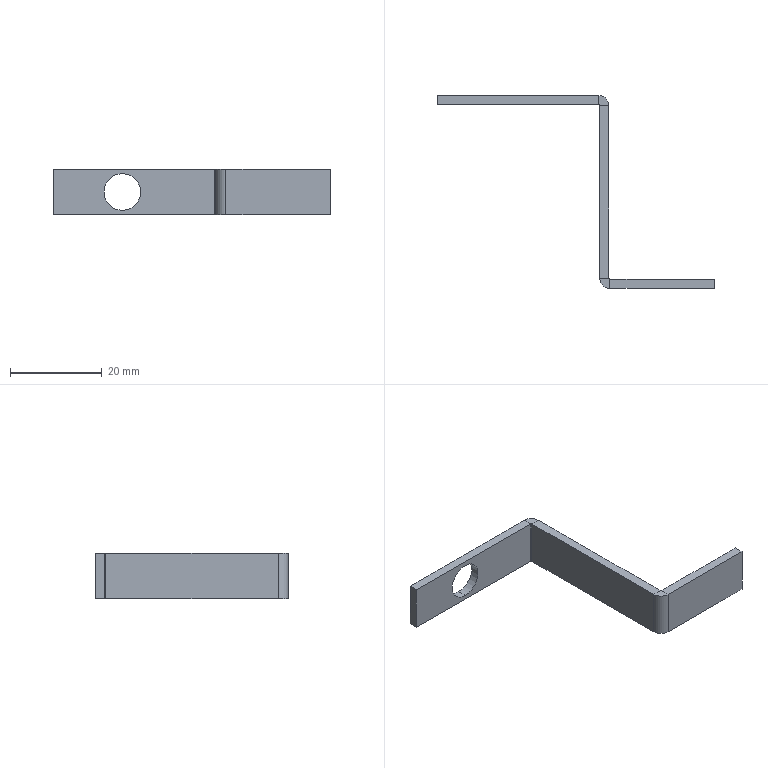Part | STEP file | Sensor support | 1 solid | 24 faces | box 60.39 x 42 x 10 mm | volume 1887 mm3 | plane 18 | cylinder 6 | commonest cylinder face diameters 0.4 x2 4.4 x2 8 x2
STEP:
#1=CARTESIAN_POINT('',(-45.39,40.,-4.));
#2=VERTEX_POINT('',#1);
#3=CARTESIAN_POINT('',(-45.39,40.,4.));
#4=VERTEX_POINT('',#3);
#5=CARTESIAN_POINT('',(-45.39,40.,0.));
#6=DIRECTION('',(0.,1.,0.));
#7=DIRECTION('',(1.,0.,0.));
#8=AXIS2_PLACEMENT_3D('',#5,#6,#7);
#9=CIRCLE('',#8,4.);
#10=EDGE_CURVE('',#2,#4,#9,.T.);
#11=ORIENTED_EDGE('',*,*,#10,.F.);
#12=CARTESIAN_POINT('',(-45.39,42.,-4.));
#13=VERTEX_POINT('',#12);
#14=CARTESIAN_POINT('',(-45.39,-0.001,-4.));
#15=DIRECTION('',(0.,1.,0.));
#16=VECTOR('',#15,1000.);
#17=LINE('',#14,#16);
#18=EDGE_CURVE('',#2,#13,#17,.T.);
#19=ORIENTED_EDGE('',*,*,#18,.T.);
#20=CARTESIAN_POINT('',(-45.39,42.,4.));
#21=VERTEX_POINT('',#20);
#22=CARTESIAN_POINT('',(-45.39,42.,0.));
#23=DIRECTION('',(0.,1.,0.));
#24=DIRECTION('',(0.,0.,1.));
#25=AXIS2_PLACEMENT_3D('',#22,#23,#24);
#26=CIRCLE('',#25,4.);
#27=EDGE_CURVE('',#13,#21,#26,.T.);
#28=ORIENTED_EDGE('',*,*,#27,.T.);
#29=CARTESIAN_POINT('',(-45.39,-0.001,4.));
#30=DIRECTION('',(0.,1.,0.));
#31=VECTOR('',#30,1000.);
#32=LINE('',#29,#31);
#33=EDGE_CURVE('',#4,#21,#32,.T.);
#34=ORIENTED_EDGE('',*,*,#33,.F.);
#35=EDGE_LOOP('',(#11,#19,#28,#34));
#36=FACE_OUTER_BOUND('',#35,.T.);
#37=CARTESIAN_POINT('',(-45.39,-0.001,0.));
#38=DIRECTION('',(0.,1.,0.));
#39=DIRECTION('',(0.,0.,1.));
#40=AXIS2_PLACEMENT_3D('',#37,#38,#39);
#41=CYLINDRICAL_SURFACE('',#40,4.);
#42=ADVANCED_FACE('',(#36),#41,.F.);
#43=CARTESIAN_POINT('',(-25.,2.2,5.));
#44=VERTEX_POINT('',#43);
#45=CARTESIAN_POINT('',(-23.,2.2,5.));
#46=VERTEX_POINT('',#45);
#47=CARTESIAN_POINT('',(-25.,2.2,5.));
#48=DIRECTION('',(1.,0.,0.));
#49=VECTOR('',#48,1000.);
#50=LINE('',#47,#49);
#51=EDGE_CURVE('',#44,#46,#50,.T.);
#52=ORIENTED_EDGE('',*,*,#51,.F.);
#53=CARTESIAN_POINT('',(-22.8,0.,5.));
#54=VERTEX_POINT('',#53);
#55=CARTESIAN_POINT('',(-22.8,2.2,5.));
#56=DIRECTION('',(0.,0.,-1.));
#57=DIRECTION('',(1.,0.,0.));
#58=AXIS2_PLACEMENT_3D('',#55,#56,#57);
#59=CIRCLE('',#58,2.2);
#60=EDGE_CURVE('',#54,#44,#59,.T.);
#61=ORIENTED_EDGE('',*,*,#60,.F.);
#62=CARTESIAN_POINT('',(-22.8,2.,5.));
#63=VERTEX_POINT('',#62);
#64=CARTESIAN_POINT('',(-22.8,2.,5.));
#65=DIRECTION('',(0.,-1.,0.));
#66=VECTOR('',#65,1000.);
#67=LINE('',#64,#66);
#68=EDGE_CURVE('',#63,#54,#67,.T.);
#69=ORIENTED_EDGE('',*,*,#68,.F.);
#70=CARTESIAN_POINT('',(-22.8,2.2,5.));
#71=DIRECTION('',(0.,0.,-1.));
#72=DIRECTION('',(1.,0.,0.));
#73=AXIS2_PLACEMENT_3D('',#70,#71,#72);
#74=CIRCLE('',#73,0.2);
#75=EDGE_CURVE('',#63,#46,#74,.T.);
#76=ORIENTED_EDGE('',*,*,#75,.T.);
#77=EDGE_LOOP('',(#52,#61,#69,#76));
#78=FACE_OUTER_BOUND('',#77,.T.);
#79=CARTESIAN_POINT('',(-25.,2.2,5.));
#80=DIRECTION('',(0.,0.,1.));
#81=DIRECTION('',(1.,0.,0.));
#82=AXIS2_PLACEMENT_3D('',#79,#80,#81);
#83=PLANE('',#82);
#84=ADVANCED_FACE('',(#78),#83,.T.);
#85=CARTESIAN_POINT('',(-25.,39.8,5.));
#86=VERTEX_POINT('',#85);
#87=CARTESIAN_POINT('',(-25.,0.,5.));
#88=DIRECTION('',(0.,1.,0.));
#89=VECTOR('',#88,1000.);
#90=LINE('',#87,#89);
#91=EDGE_CURVE('',#44,#86,#90,.T.);
#92=ORIENTED_EDGE('',*,*,#91,.F.);
#93=ORIENTED_EDGE('',*,*,#51,.T.);
#94=CARTESIAN_POINT('',(-23.,39.8,5.));
#95=VERTEX_POINT('',#94);
#96=CARTESIAN_POINT('',(-23.,0.,5.));
#97=DIRECTION('',(0.,1.,0.));
#98=VECTOR('',#97,1000.);
#99=LINE('',#96,#98);
#100=EDGE_CURVE('',#46,#95,#99,.T.);
#101=ORIENTED_EDGE('',*,*,#100,.T.);
#102=CARTESIAN_POINT('',(-23.,39.8,5.));
#103=DIRECTION('',(-1.,0.,0.));
#104=VECTOR('',#103,1000.);
#105=LINE('',#102,#104);
#106=EDGE_CURVE('',#95,#86,#105,.T.);
#107=ORIENTED_EDGE('',*,*,#106,.T.);
#108=EDGE_LOOP('',(#92,#93,#101,#107));
#109=FACE_OUTER_BOUND('',#108,.T.);
#110=CARTESIAN_POINT('',(-22.8,2.,5.));
#111=DIRECTION('',(0.,0.,1.));
#112=DIRECTION('',(1.,0.,0.));
#113=AXIS2_PLACEMENT_3D('',#110,#111,#112);
#114=PLANE('',#113);
#115=ADVANCED_FACE('',(#109),#114,.T.);
#116=CARTESIAN_POINT('',(-22.8,0.,-5.));
#117=VERTEX_POINT('',#116);
#118=CARTESIAN_POINT('',(-22.8,2.,-5.));
#119=VERTEX_POINT('',#118);
#120=CARTESIAN_POINT('',(-22.8,0.,-5.));
#121=DIRECTION('',(0.,1.,0.));
#122=VECTOR('',#121,1000.);
#123=LINE('',#120,#122);
#124=EDGE_CURVE('',#117,#119,#123,.T.);
#125=ORIENTED_EDGE('',*,*,#124,.F.);
#126=CARTESIAN_POINT('',(-25.,2.2,-5.));
#127=VERTEX_POINT('',#126);
#128=CARTESIAN_POINT('',(-22.8,2.2,-5.));
#129=DIRECTION('',(0.,0.,-1.));
#130=DIRECTION('',(1.,0.,0.));
#131=AXIS2_PLACEMENT_3D('',#128,#129,#130);
#132=CIRCLE('',#131,2.2);
#133=EDGE_CURVE('',#117,#127,#132,.T.);
#134=ORIENTED_EDGE('',*,*,#133,.T.);
#135=CARTESIAN_POINT('',(-23.,2.2,-5.));
#136=VERTEX_POINT('',#135);
#137=CARTESIAN_POINT('',(-23.,2.2,-5.));
#138=DIRECTION('',(-1.,0.,0.));
#139=VECTOR('',#138,1000.);
#140=LINE('',#137,#139);
#141=EDGE_CURVE('',#136,#127,#140,.T.);
#142=ORIENTED_EDGE('',*,*,#141,.F.);
#143=CARTESIAN_POINT('',(-22.8,2.2,-5.));
#144=DIRECTION('',(0.,0.,-1.));
#145=DIRECTION('',(1.,0.,0.));
#146=AXIS2_PLACEMENT_3D('',#143,#144,#145);
#147=CIRCLE('',#146,0.2);
#148=EDGE_CURVE('',#119,#136,#147,.T.);
#149=ORIENTED_EDGE('',*,*,#148,.F.);
#150=EDGE_LOOP('',(#125,#134,#142,#149));
#151=FACE_OUTER_BOUND('',#150,.T.);
#152=CARTESIAN_POINT('',(-22.8,0.,-5.));
#153=DIRECTION('',(0.,0.,-1.));
#154=DIRECTION('',(-1.,0.,0.));
#155=AXIS2_PLACEMENT_3D('',#152,#153,#154);
#156=PLANE('',#155);
#157=ADVANCED_FACE('',(#151),#156,.T.);
#158=CARTESIAN_POINT('',(0.,0.,-5.));
#159=VERTEX_POINT('',#158);
#160=CARTESIAN_POINT('',(0.,0.,-5.));
#161=DIRECTION('',(-1.,0.,0.));
#162=VECTOR('',#161,1000.);
#163=LINE('',#160,#162);
#164=EDGE_CURVE('',#159,#117,#163,.T.);
#165=ORIENTED_EDGE('',*,*,#164,.T.);
#166=ORIENTED_EDGE('',*,*,#124,.T.);
#167=CARTESIAN_POINT('',(0.,2.,-5.));
#168=VERTEX_POINT('',#167);
#169=CARTESIAN_POINT('',(0.,2.,-5.));
#170=DIRECTION('',(-1.,0.,0.));
#171=VECTOR('',#170,1000.);
#172=LINE('',#169,#171);
#173=EDGE_CURVE('',#168,#119,#172,.T.);
#174=ORIENTED_EDGE('',*,*,#173,.F.);
#175=CARTESIAN_POINT('',(0.,2.,-5.));
#176=DIRECTION('',(0.,-1.,0.));
#177=VECTOR('',#176,1000.);
#178=LINE('',#175,#177);
#179=EDGE_CURVE('',#168,#159,#178,.T.);
#180=ORIENTED_EDGE('',*,*,#179,.T.);
#181=EDGE_LOOP('',(#165,#166,#174,#180));
#182=FACE_OUTER_BOUND('',#181,.T.);
#183=CARTESIAN_POINT('',(-23.,2.2,-5.));
#184=DIRECTION('',(0.,0.,-1.));
#185=DIRECTION('',(-1.,0.,0.));
#186=AXIS2_PLACEMENT_3D('',#183,#184,#185);
#187=PLANE('',#186);
#188=ADVANCED_FACE('',(#182),#187,.T.);
#189=CARTESIAN_POINT('',(-25.2,40.,5.));
#190=VERTEX_POINT('',#189);
#191=CARTESIAN_POINT('',(-25.2,42.,5.));
#192=VERTEX_POINT('',#191);
#193=CARTESIAN_POINT('',(-25.2,40.,5.));
#194=DIRECTION('',(0.,1.,0.));
#195=VECTOR('',#194,1000.);
#196=LINE('',#193,#195);
#197=EDGE_CURVE('',#190,#192,#196,.T.);
#198=ORIENTED_EDGE('',*,*,#197,.F.);
#199=CARTESIAN_POINT('',(-25.2,39.8,5.));
#200=DIRECTION('',(0.,0.,1.));
#201=DIRECTION('',(-1.,0.,0.));
#202=AXIS2_PLACEMENT_3D('',#199,#200,#201);
#203=CIRCLE('',#202,0.2);
#204=EDGE_CURVE('',#86,#190,#203,.T.);
#205=ORIENTED_EDGE('',*,*,#204,.F.);
#206=ORIENTED_EDGE('',*,*,#106,.F.);
#207=CARTESIAN_POINT('',(-25.2,39.8,5.));
#208=DIRECTION('',(0.,0.,1.));
#209=DIRECTION('',(1.,0.,0.));
#210=AXIS2_PLACEMENT_3D('',#207,#208,#209);
#211=CIRCLE('',#210,2.2);
#212=EDGE_CURVE('',#95,#192,#211,.T.);
#213=ORIENTED_EDGE('',*,*,#212,.T.);
#214=EDGE_LOOP('',(#198,#205,#206,#213));
#215=FACE_OUTER_BOUND('',#214,.T.);
#216=CARTESIAN_POINT('',(-25.2,40.,5.));
#217=DIRECTION('',(0.,0.,1.));
#218=DIRECTION('',(1.,0.,0.));
#219=AXIS2_PLACEMENT_3D('',#216,#217,#218);
#220=PLANE('',#219);
#221=ADVANCED_FACE('',(#215),#220,.T.);
#222=CARTESIAN_POINT('',(-60.39,40.,5.));
#223=VERTEX_POINT('',#222);
#224=CARTESIAN_POINT('',(-25.,40.,5.));
#225=DIRECTION('',(-1.,0.,0.));
#226=VECTOR('',#225,1000.);
#227=LINE('',#224,#226);
#228=EDGE_CURVE('',#190,#223,#227,.T.);
#229=ORIENTED_EDGE('',*,*,#228,.F.);
#230=ORIENTED_EDGE('',*,*,#197,.T.);
#231=CARTESIAN_POINT('',(-60.39,42.,5.));
#232=VERTEX_POINT('',#231);
#233=CARTESIAN_POINT('',(-25.,42.,5.));
#234=DIRECTION('',(-1.,0.,0.));
#235=VECTOR('',#234,1000.);
#236=LINE('',#233,#235);
#237=EDGE_CURVE('',#192,#232,#236,.T.);
#238=ORIENTED_EDGE('',*,*,#237,.T.);
#239=CARTESIAN_POINT('',(-60.39,40.,5.));
#240=DIRECTION('',(0.,1.,0.));
#241=VECTOR('',#240,1000.);
#242=LINE('',#239,#241);
#243=EDGE_CURVE('',#223,#232,#242,.T.);
#244=ORIENTED_EDGE('',*,*,#243,.F.);
#245=EDGE_LOOP('',(#229,#230,#238,#244));
#246=FACE_OUTER_BOUND('',#245,.T.);
#247=CARTESIAN_POINT('',(-23.,39.8,5.));
#248=DIRECTION('',(0.,0.,1.));
#249=DIRECTION('',(1.,0.,0.));
#250=AXIS2_PLACEMENT_3D('',#247,#248,#249);
#251=PLANE('',#250);
#252=ADVANCED_FACE('',(#246),#251,.T.);
#253=CARTESIAN_POINT('',(-25.,39.8,-5.));
#254=VERTEX_POINT('',#253);
#255=CARTESIAN_POINT('',(-23.,39.8,-5.));
#256=VERTEX_POINT('',#255);
#257=CARTESIAN_POINT('',(-25.,39.8,-5.));
#258=DIRECTION('',(1.,0.,0.));
#259=VECTOR('',#258,1000.);
#260=LINE('',#257,#259);
#261=EDGE_CURVE('',#254,#256,#260,.T.);
#262=ORIENTED_EDGE('',*,*,#261,.F.);
#263=CARTESIAN_POINT('',(-25.2,40.,-5.));
#264=VERTEX_POINT('',#263);
#265=CARTESIAN_POINT('',(-25.2,39.8,-5.));
#266=DIRECTION('',(0.,0.,1.));
#267=DIRECTION('',(-1.,0.,0.));
#268=AXIS2_PLACEMENT_3D('',#265,#266,#267);
#269=CIRCLE('',#268,0.2);
#270=EDGE_CURVE('',#254,#264,#269,.T.);
#271=ORIENTED_EDGE('',*,*,#270,.T.);
#272=CARTESIAN_POINT('',(-25.2,42.,-5.));
#273=VERTEX_POINT('',#272);
#274=CARTESIAN_POINT('',(-25.2,42.,-5.));
#275=DIRECTION('',(0.,-1.,0.));
#276=VECTOR('',#275,1000.);
#277=LINE('',#274,#276);
#278=EDGE_CURVE('',#273,#264,#277,.T.);
#279=ORIENTED_EDGE('',*,*,#278,.F.);
#280=CARTESIAN_POINT('',(-25.2,39.8,-5.));
#281=DIRECTION('',(0.,0.,1.));
#282=DIRECTION('',(1.,0.,0.));
#283=AXIS2_PLACEMENT_3D('',#280,#281,#282);
#284=CIRCLE('',#283,2.2);
#285=EDGE_CURVE('',#256,#273,#284,.T.);
#286=ORIENTED_EDGE('',*,*,#285,.F.);
#287=EDGE_LOOP('',(#262,#271,#279,#286));
#288=FACE_OUTER_BOUND('',#287,.T.);
#289=CARTESIAN_POINT('',(-25.,39.8,-5.));
#290=DIRECTION('',(0.,0.,-1.));
#291=DIRECTION('',(-1.,0.,0.));
#292=AXIS2_PLACEMENT_3D('',#289,#290,#291);
#293=PLANE('',#292);
#294=ADVANCED_FACE('',(#288),#293,.T.);
#295=CARTESIAN_POINT('',(-25.,0.,-5.));
#296=DIRECTION('',(0.,1.,0.));
#297=VECTOR('',#296,1000.);
#298=LINE('',#295,#297);
#299=EDGE_CURVE('',#127,#254,#298,.T.);
#300=ORIENTED_EDGE('',*,*,#299,.T.);
#301=ORIENTED_EDGE('',*,*,#261,.T.);
#302=CARTESIAN_POINT('',(-23.,0.,-5.));
#303=DIRECTION('',(0.,1.,0.));
#304=VECTOR('',#303,1000.);
#305=LINE('',#302,#304);
#306=EDGE_CURVE('',#136,#256,#305,.T.);
#307=ORIENTED_EDGE('',*,*,#306,.F.);
#308=ORIENTED_EDGE('',*,*,#141,.T.);
#309=EDGE_LOOP('',(#300,#301,#307,#308));
#310=FACE_OUTER_BOUND('',#309,.T.);
#311=CARTESIAN_POINT('',(-25.2,42.,-5.));
#312=DIRECTION('',(0.,0.,-1.));
#313=DIRECTION('',(-1.,0.,0.));
#314=AXIS2_PLACEMENT_3D('',#311,#312,#313);
#315=PLANE('',#314);
#316=ADVANCED_FACE('',(#310),#315,.T.);
#317=CARTESIAN_POINT('',(-45.39,42.,0.));
#318=DIRECTION('',(0.,1.,0.));
#319=DIRECTION('',(0.,0.,1.));
#320=AXIS2_PLACEMENT_3D('',#317,#318,#319);
#321=CIRCLE('',#320,4.);
#322=EDGE_CURVE('',#21,#13,#321,.T.);
#323=ORIENTED_EDGE('',*,*,#322,.F.);
#324=ORIENTED_EDGE('',*,*,#27,.F.);
#325=EDGE_LOOP('',(#323,#324));
#326=FACE_BOUND('',#325,.T.);
#327=CARTESIAN_POINT('',(-60.39,42.,-5.));
#328=VERTEX_POINT('',#327);
#329=CARTESIAN_POINT('',(-25.,42.,-5.));
#330=DIRECTION('',(-1.,0.,0.));
#331=VECTOR('',#330,1000.);
#332=LINE('',#329,#331);
#333=EDGE_CURVE('',#273,#328,#332,.T.);
#334=ORIENTED_EDGE('',*,*,#333,.T.);
#335=CARTESIAN_POINT('',(-60.39,42.,5.));
#336=DIRECTION('',(0.,0.,-1.));
#337=VECTOR('',#336,1000.);
#338=LINE('',#335,#337);
#339=EDGE_CURVE('',#232,#328,#338,.T.);
#340=ORIENTED_EDGE('',*,*,#339,.F.);
#341=ORIENTED_EDGE('',*,*,#237,.F.);
#342=CARTESIAN_POINT('',(-25.2,42.,5.));
#343=DIRECTION('',(0.,0.,-1.));
#344=VECTOR('',#343,1000.);
#345=LINE('',#342,#344);
#346=EDGE_CURVE('',#192,#273,#345,.T.);
#347=ORIENTED_EDGE('',*,*,#346,.T.);
#348=EDGE_LOOP('',(#334,#340,#341,#347));
#349=FACE_OUTER_BOUND('',#348,.T.);
#350=CARTESIAN_POINT('',(-25.,42.,5.));
#351=DIRECTION('',(0.,-1.,0.));
#352=DIRECTION('',(1.,0.,0.));
#353=AXIS2_PLACEMENT_3D('',#350,#351,#352);
#354=PLANE('',#353);
#355=ADVANCED_FACE('',(#326,#349),#354,.F.);
#356=CARTESIAN_POINT('',(-60.39,40.,-5.));
#357=VERTEX_POINT('',#356);
#358=CARTESIAN_POINT('',(-60.39,40.,-5.));
#359=DIRECTION('',(0.,1.,0.));
#360=VECTOR('',#359,1000.);
#361=LINE('',#358,#360);
#362=EDGE_CURVE('',#357,#328,#361,.T.);
#363=ORIENTED_EDGE('',*,*,#362,.F.);
#364=CARTESIAN_POINT('',(-60.39,40.,5.));
#365=DIRECTION('',(0.,0.,-1.));
#366=VECTOR('',#365,1000.);
#367=LINE('',#364,#366);
#368=EDGE_CURVE('',#223,#357,#367,.T.);
#369=ORIENTED_EDGE('',*,*,#368,.F.);
#370=ORIENTED_EDGE('',*,*,#243,.T.);
#371=ORIENTED_EDGE('',*,*,#339,.T.);
#372=EDGE_LOOP('',(#363,#369,#370,#371));
#373=FACE_OUTER_BOUND('',#372,.T.);
#374=CARTESIAN_POINT('',(-60.39,40.,5.));
#375=DIRECTION('',(-1.,0.,0.));
#376=DIRECTION('',(0.,0.,1.));
#377=AXIS2_PLACEMENT_3D('',#374,#375,#376);
#378=PLANE('',#377);
#379=ADVANCED_FACE('',(#373),#378,.T.);
#380=CARTESIAN_POINT('',(-45.39,40.,0.));
#381=DIRECTION('',(0.,1.,0.));
#382=DIRECTION('',(1.,0.,0.));
#383=AXIS2_PLACEMENT_3D('',#380,#381,#382);
#384=CIRCLE('',#383,4.);
#385=EDGE_CURVE('',#4,#2,#384,.T.);
#386=ORIENTED_EDGE('',*,*,#385,.T.);
#387=ORIENTED_EDGE('',*,*,#10,.T.);
#388=EDGE_LOOP('',(#386,#387));
#389=FACE_BOUND('',#388,.T.);
#390=CARTESIAN_POINT('',(-25.,40.,-5.));
#391=DIRECTION('',(-1.,0.,0.));
#392=VECTOR('',#391,1000.);
#393=LINE('',#390,#392);
#394=EDGE_CURVE('',#264,#357,#393,.T.);
#395=ORIENTED_EDGE('',*,*,#394,.F.);
#396=CARTESIAN_POINT('',(-25.2,40.,5.));
#397=DIRECTION('',(0.,0.,-1.));
#398=VECTOR('',#397,1000.);
#399=LINE('',#396,#398);
#400=EDGE_CURVE('',#190,#264,#399,.T.);
#401=ORIENTED_EDGE('',*,*,#400,.F.);
#402=ORIENTED_EDGE('',*,*,#228,.T.);
#403=ORIENTED_EDGE('',*,*,#368,.T.);
#404=EDGE_LOOP('',(#395,#401,#402,#403));
#405=FACE_OUTER_BOUND('',#404,.T.);
#406=CARTESIAN_POINT('',(-25.,40.,5.));
#407=DIRECTION('',(0.,-1.,0.));
#408=DIRECTION('',(1.,0.,0.));
#409=AXIS2_PLACEMENT_3D('',#406,#407,#408);
#410=PLANE('',#409);
#411=ADVANCED_FACE('',(#389,#405),#410,.T.);
#412=ORIENTED_EDGE('',*,*,#270,.F.);
#413=CARTESIAN_POINT('',(-25.,39.8,5.));
#414=DIRECTION('',(0.,0.,-1.));
#415=VECTOR('',#414,1000.);
#416=LINE('',#413,#415);
#417=EDGE_CURVE('',#86,#254,#416,.T.);
#418=ORIENTED_EDGE('',*,*,#417,.F.);
#419=ORIENTED_EDGE('',*,*,#204,.T.);
#420=ORIENTED_EDGE('',*,*,#400,.T.);
#421=EDGE_LOOP('',(#412,#418,#419,#420));
#422=FACE_OUTER_BOUND('',#421,.T.);
#423=CARTESIAN_POINT('',(-25.2,39.8,5.));
#424=DIRECTION('',(0.,0.,-1.));
#425=DIRECTION('',(-1.,0.,0.));
#426=AXIS2_PLACEMENT_3D('',#423,#424,#425);
#427=CYLINDRICAL_SURFACE('',#426,0.2);
#428=ADVANCED_FACE('',(#422),#427,.F.);
#429=ORIENTED_EDGE('',*,*,#299,.F.);
#430=CARTESIAN_POINT('',(-25.,2.2,5.));
#431=DIRECTION('',(0.,0.,-1.));
#432=VECTOR('',#431,1000.);
#433=LINE('',#430,#432);
#434=EDGE_CURVE('',#44,#127,#433,.T.);
#435=ORIENTED_EDGE('',*,*,#434,.F.);
#436=ORIENTED_EDGE('',*,*,#91,.T.);
#437=ORIENTED_EDGE('',*,*,#417,.T.);
#438=EDGE_LOOP('',(#429,#435,#436,#437));
#439=FACE_OUTER_BOUND('',#438,.T.);
#440=CARTESIAN_POINT('',(-25.,0.,5.));
#441=DIRECTION('',(-1.,0.,0.));
#442=DIRECTION('',(0.,0.,1.));
#443=AXIS2_PLACEMENT_3D('',#440,#441,#442);
#444=PLANE('',#443);
#445=ADVANCED_FACE('',(#439),#444,.T.);
#446=ORIENTED_EDGE('',*,*,#133,.F.);
#447=CARTESIAN_POINT('',(-22.8,0.,5.));
#448=DIRECTION('',(0.,0.,-1.));
#449=VECTOR('',#448,1000.);
#450=LINE('',#447,#449);
#451=EDGE_CURVE('',#54,#117,#450,.T.);
#452=ORIENTED_EDGE('',*,*,#451,.F.);
#453=ORIENTED_EDGE('',*,*,#60,.T.);
#454=ORIENTED_EDGE('',*,*,#434,.T.);
#455=EDGE_LOOP('',(#446,#452,#453,#454));
#456=FACE_OUTER_BOUND('',#455,.T.);
#457=CARTESIAN_POINT('',(-22.8,2.2,5.));
#458=DIRECTION('',(0.,0.,-1.));
#459=DIRECTION('',(-1.,0.,0.));
#460=AXIS2_PLACEMENT_3D('',#457,#458,#459);
#461=CYLINDRICAL_SURFACE('',#460,2.2);
#462=ADVANCED_FACE('',(#456),#461,.T.);
#463=ORIENTED_EDGE('',*,*,#164,.F.);
#464=CARTESIAN_POINT('',(0.,0.,5.));
#465=VERTEX_POINT('',#464);
#466=CARTESIAN_POINT('',(0.,0.,5.));
#467=DIRECTION('',(0.,0.,-1.));
#468=VECTOR('',#467,1000.);
#469=LINE('',#466,#468);
#470=EDGE_CURVE('',#465,#159,#469,.T.);
#471=ORIENTED_EDGE('',*,*,#470,.F.);
#472=CARTESIAN_POINT('',(0.,0.,5.));
#473=DIRECTION('',(-1.,0.,0.));
#474=VECTOR('',#473,1000.);
#475=LINE('',#472,#474);
#476=EDGE_CURVE('',#465,#54,#475,.T.);
#477=ORIENTED_EDGE('',*,*,#476,.T.);
#478=ORIENTED_EDGE('',*,*,#451,.T.);
#479=EDGE_LOOP('',(#463,#471,#477,#478));
#480=FACE_OUTER_BOUND('',#479,.T.);
#481=CARTESIAN_POINT('',(0.,0.,5.));
#482=DIRECTION('',(0.,-1.,0.));
#483=DIRECTION('',(1.,0.,0.));
#484=AXIS2_PLACEMENT_3D('',#481,#482,#483);
#485=PLANE('',#484);
#486=ADVANCED_FACE('',(#480),#485,.T.);
#487=ORIENTED_EDGE('',*,*,#179,.F.);
#488=CARTESIAN_POINT('',(0.,2.,5.));
#489=VERTEX_POINT('',#488);
#490=CARTESIAN_POINT('',(0.,2.,5.));
#491=DIRECTION('',(0.,0.,-1.));
#492=VECTOR('',#491,1000.);
#493=LINE('',#490,#492);
#494=EDGE_CURVE('',#489,#168,#493,.T.);
#495=ORIENTED_EDGE('',*,*,#494,.F.);
#496=CARTESIAN_POINT('',(0.,2.,5.));
#497=DIRECTION('',(0.,-1.,0.));
#498=VECTOR('',#497,1000.);
#499=LINE('',#496,#498);
#500=EDGE_CURVE('',#489,#465,#499,.T.);
#501=ORIENTED_EDGE('',*,*,#500,.T.);
#502=ORIENTED_EDGE('',*,*,#470,.T.);
#503=EDGE_LOOP('',(#487,#495,#501,#502));
#504=FACE_OUTER_BOUND('',#503,.T.);
#505=CARTESIAN_POINT('',(0.,2.,5.));
#506=DIRECTION('',(1.,0.,0.));
#507=DIRECTION('',(0.,1.,0.));
#508=AXIS2_PLACEMENT_3D('',#505,#506,#507);
#509=PLANE('',#508);
#510=ADVANCED_FACE('',(#504),#509,.T.);
#511=ORIENTED_EDGE('',*,*,#173,.T.);
#512=CARTESIAN_POINT('',(-22.8,2.,5.));
#513=DIRECTION('',(0.,0.,-1.));
#514=VECTOR('',#513,1000.);
#515=LINE('',#512,#514);
#516=EDGE_CURVE('',#63,#119,#515,.T.);
#517=ORIENTED_EDGE('',*,*,#516,.F.);
#518=CARTESIAN_POINT('',(0.,2.,5.));
#519=DIRECTION('',(-1.,0.,0.));
#520=VECTOR('',#519,1000.);
#521=LINE('',#518,#520);
#522=EDGE_CURVE('',#489,#63,#521,.T.);
#523=ORIENTED_EDGE('',*,*,#522,.F.);
#524=ORIENTED_EDGE('',*,*,#494,.T.);
#525=EDGE_LOOP('',(#511,#517,#523,#524));
#526=FACE_OUTER_BOUND('',#525,.T.);
#527=CARTESIAN_POINT('',(0.,2.,5.));
#528=DIRECTION('',(0.,-1.,0.));
#529=DIRECTION('',(1.,0.,0.));
#530=AXIS2_PLACEMENT_3D('',#527,#528,#529);
#531=PLANE('',#530);
#532=ADVANCED_FACE('',(#526),#531,.F.);
#533=ORIENTED_EDGE('',*,*,#148,.T.);
#534=CARTESIAN_POINT('',(-23.,2.2,5.));
#535=DIRECTION('',(0.,0.,-1.));
#536=VECTOR('',#535,1000.);
#537=LINE('',#534,#536);
#538=EDGE_CURVE('',#46,#136,#537,.T.);
#539=ORIENTED_EDGE('',*,*,#538,.F.);
#540=ORIENTED_EDGE('',*,*,#75,.F.);
#541=ORIENTED_EDGE('',*,*,#516,.T.);
#542=EDGE_LOOP('',(#533,#539,#540,#541));
#543=FACE_OUTER_BOUND('',#542,.T.);
#544=CARTESIAN_POINT('',(-22.8,2.2,5.));
#545=DIRECTION('',(0.,0.,-1.));
#546=DIRECTION('',(-1.,0.,0.));
#547=AXIS2_PLACEMENT_3D('',#544,#545,#546);
#548=CYLINDRICAL_SURFACE('',#547,0.2);
#549=ADVANCED_FACE('',(#543),#548,.F.);
#550=ORIENTED_EDGE('',*,*,#306,.T.);
#551=CARTESIAN_POINT('',(-23.,39.8,5.));
#552=DIRECTION('',(0.,0.,-1.));
#553=VECTOR('',#552,1000.);
#554=LINE('',#551,#553);
#555=EDGE_CURVE('',#95,#256,#554,.T.);
#556=ORIENTED_EDGE('',*,*,#555,.F.);
#557=ORIENTED_EDGE('',*,*,#100,.F.);
#558=ORIENTED_EDGE('',*,*,#538,.T.);
#559=EDGE_LOOP('',(#550,#556,#557,#558));
#560=FACE_OUTER_BOUND('',#559,.T.);
#561=CARTESIAN_POINT('',(-23.,0.,5.));
#562=DIRECTION('',(-1.,0.,0.));
#563=DIRECTION('',(0.,0.,1.));
#564=AXIS2_PLACEMENT_3D('',#561,#562,#563);
#565=PLANE('',#564);
#566=ADVANCED_FACE('',(#560),#565,.F.);
#567=ORIENTED_EDGE('',*,*,#285,.T.);
#568=ORIENTED_EDGE('',*,*,#346,.F.);
#569=ORIENTED_EDGE('',*,*,#212,.F.);
#570=ORIENTED_EDGE('',*,*,#555,.T.);
#571=EDGE_LOOP('',(#567,#568,#569,#570));
#572=FACE_OUTER_BOUND('',#571,.T.);
#573=CARTESIAN_POINT('',(-25.2,39.8,5.));
#574=DIRECTION('',(0.,0.,-1.));
#575=DIRECTION('',(-1.,0.,0.));
#576=AXIS2_PLACEMENT_3D('',#573,#574,#575);
#577=CYLINDRICAL_SURFACE('',#576,2.2);
#578=ADVANCED_FACE('',(#572),#577,.T.);
#579=ORIENTED_EDGE('',*,*,#522,.T.);
#580=ORIENTED_EDGE('',*,*,#68,.T.);
#581=ORIENTED_EDGE('',*,*,#476,.F.);
#582=ORIENTED_EDGE('',*,*,#500,.F.);
#583=EDGE_LOOP('',(#579,#580,#581,#582));
#584=FACE_OUTER_BOUND('',#583,.T.);
#585=CARTESIAN_POINT('',(-25.2,39.8,5.));
#586=DIRECTION('',(0.,0.,-1.));
#587=DIRECTION('',(-1.,0.,0.));
#588=AXIS2_PLACEMENT_3D('',#585,#586,#587);
#589=PLANE('',#588);
#590=ADVANCED_FACE('',(#584),#589,.F.);
#591=ORIENTED_EDGE('',*,*,#333,.F.);
#592=ORIENTED_EDGE('',*,*,#278,.T.);
#593=ORIENTED_EDGE('',*,*,#394,.T.);
#594=ORIENTED_EDGE('',*,*,#362,.T.);
#595=EDGE_LOOP('',(#591,#592,#593,#594));
#596=FACE_OUTER_BOUND('',#595,.T.);
#597=CARTESIAN_POINT('',(-25.2,39.8,-5.));
#598=DIRECTION('',(0.,0.,-1.));
#599=DIRECTION('',(-1.,0.,0.));
#600=AXIS2_PLACEMENT_3D('',#597,#598,#599);
#601=PLANE('',#600);
#602=ADVANCED_FACE('',(#596),#601,.T.);
#603=ORIENTED_EDGE('',*,*,#18,.F.);
#604=ORIENTED_EDGE('',*,*,#385,.F.);
#605=ORIENTED_EDGE('',*,*,#33,.T.);
#606=ORIENTED_EDGE('',*,*,#322,.T.);
#607=EDGE_LOOP('',(#603,#604,#605,#606));
#608=FACE_OUTER_BOUND('',#607,.T.);
#609=CARTESIAN_POINT('',(-45.39,-0.001,0.));
#610=DIRECTION('',(0.,1.,0.));
#611=DIRECTION('',(0.,0.,1.));
#612=AXIS2_PLACEMENT_3D('',#609,#610,#611);
#613=CYLINDRICAL_SURFACE('',#612,4.);
#614=ADVANCED_FACE('',(#608),#613,.F.);
#615=CLOSED_SHELL('',(#42,#84,#115,#157,#188,#221,#252,#294,#316,#355,#379,#411,#428,#445,#462,#486,#510,#532,#549,#566,#578,#590,#602,#614));
#616=MANIFOLD_SOLID_BREP('',#615);
#617=CARTESIAN_POINT('',(0.,0.,0.));
#618=DIRECTION('',(0.,0.,1.));
#619=DIRECTION('',(1.,0.,0.));
#620=AXIS2_PLACEMENT_3D('',#617,#618,#619);
#621=(LENGTH_UNIT()NAMED_UNIT(*)SI_UNIT(.MILLI.,.METRE.));
#622=UNCERTAINTY_MEASURE_WITH_UNIT(LENGTH_MEASURE(0.00001),#621,'','');
#623=(NAMED_UNIT(*)PLANE_ANGLE_UNIT()SI_UNIT($,.RADIAN.));
#624=(NAMED_UNIT(*)SI_UNIT($,.STERADIAN.)SOLID_ANGLE_UNIT());
#625=(GEOMETRIC_REPRESENTATION_CONTEXT(3)GLOBAL_UNCERTAINTY_ASSIGNED_CONTEXT((#622))GLOBAL_UNIT_ASSIGNED_CONTEXT((#621,#623,#624))REPRESENTATION_CONTEXT('',''));
#626=ADVANCED_BREP_SHAPE_REPRESENTATION('',(#616,#620),#625);